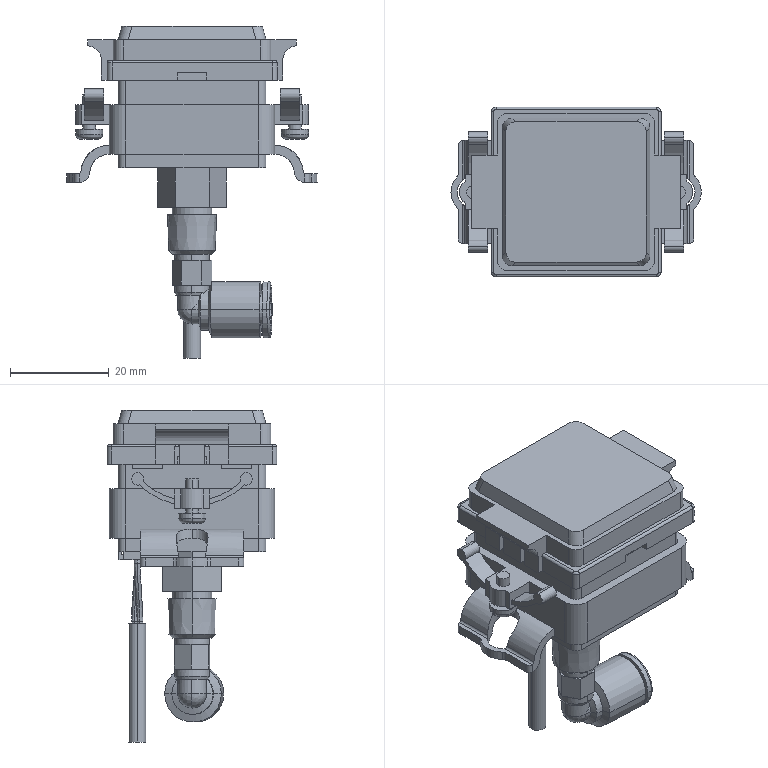Part | SolidWorks | 8 solids | 563 faces | box 50.8 x 34.5 x 67.4 mm | volume 31977 mm3 | plane 303 | cylinder 196 | cone 38 | torus 18 | spline 6 | sphere 2 | commonest cylinder face diameters 1 x30 2 x16 2.5 x16 1.2 x12 2.6 x12 3 x12